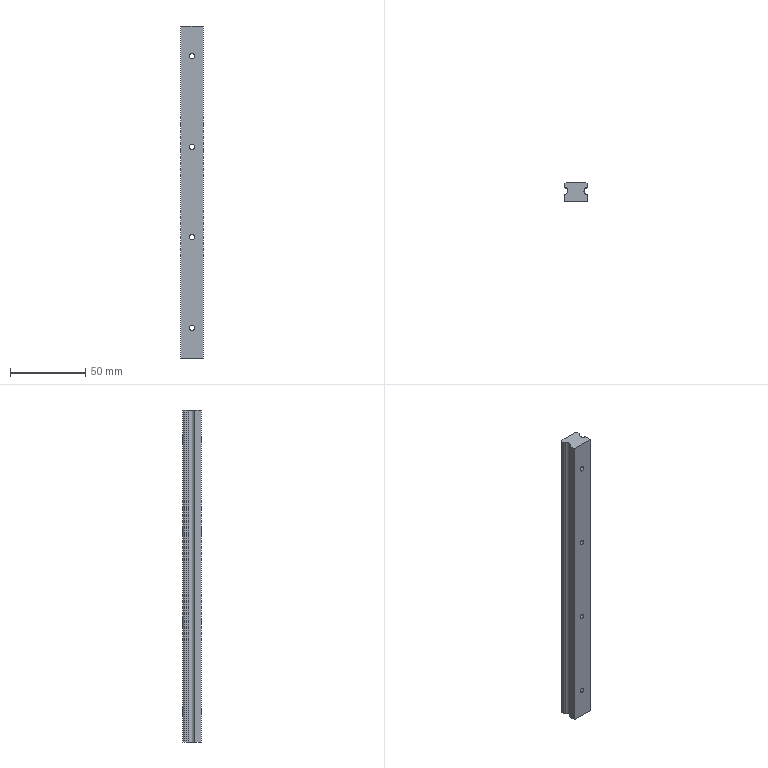Part | STEP file | rail1_SXR24_220 | 1 solid | 35 faces | box 15 x 12.5 x 220 mm | volume 36709 mm3 | cylinder 21 | plane 14 | commonest cylinder face diameters 3.5 x8 6 x8 4.4 x3 3 x2